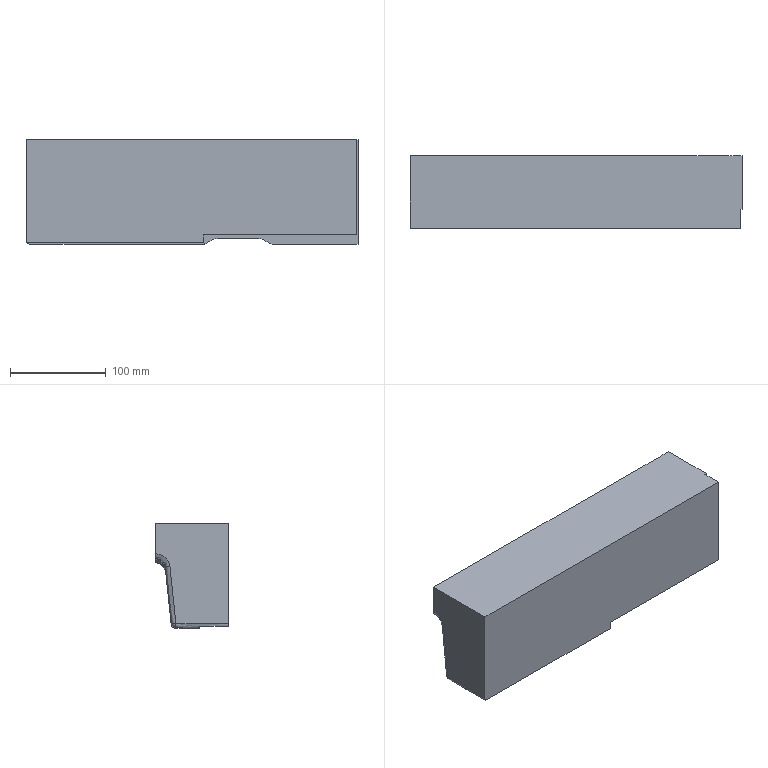Part | NX | features solid 2 | 1 solid | 75 faces | box 347.1 x 75.986 x 109.55 mm | volume 2490293 mm3 | spline 60 | plane 14 | sphere 1